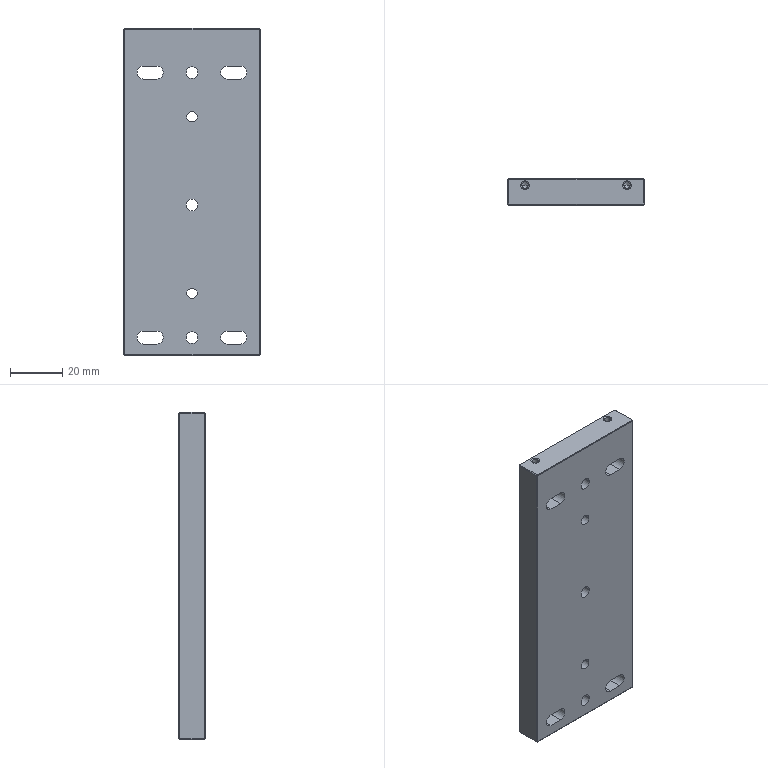Part | NX | 1 solid | 77 faces | box 52 x 10 x 125 mm | volume 61896 mm3 | cylinder 36 | plane 29 | cone 12 | commonest cylinder face diameters 5 x12 2.5 x8 4.5 x6 8 x6 4 x4